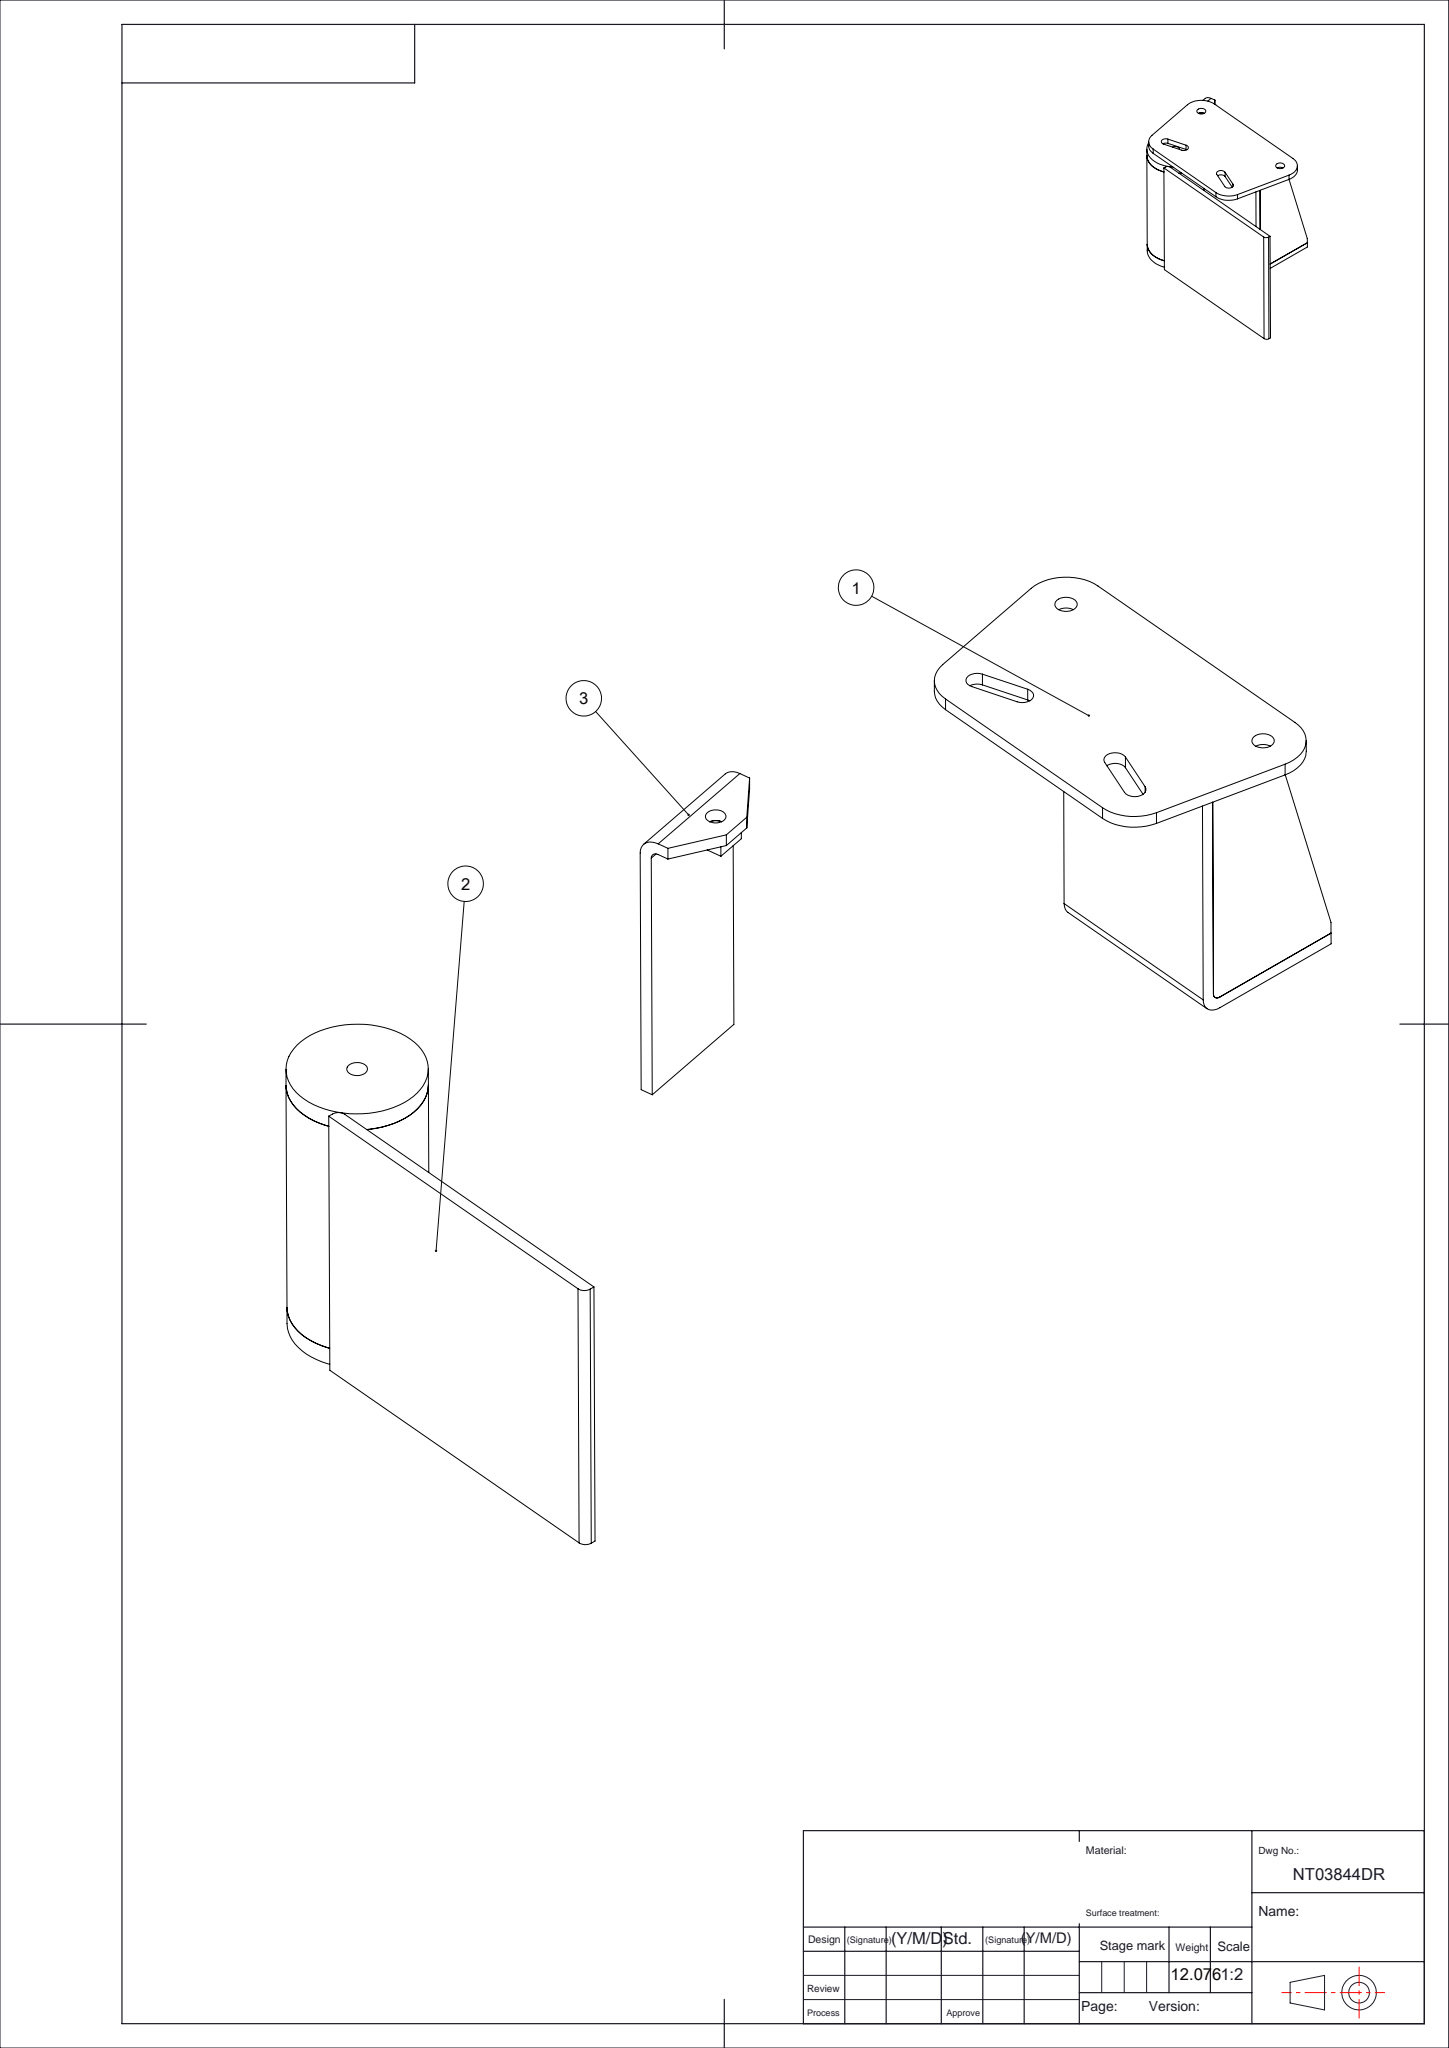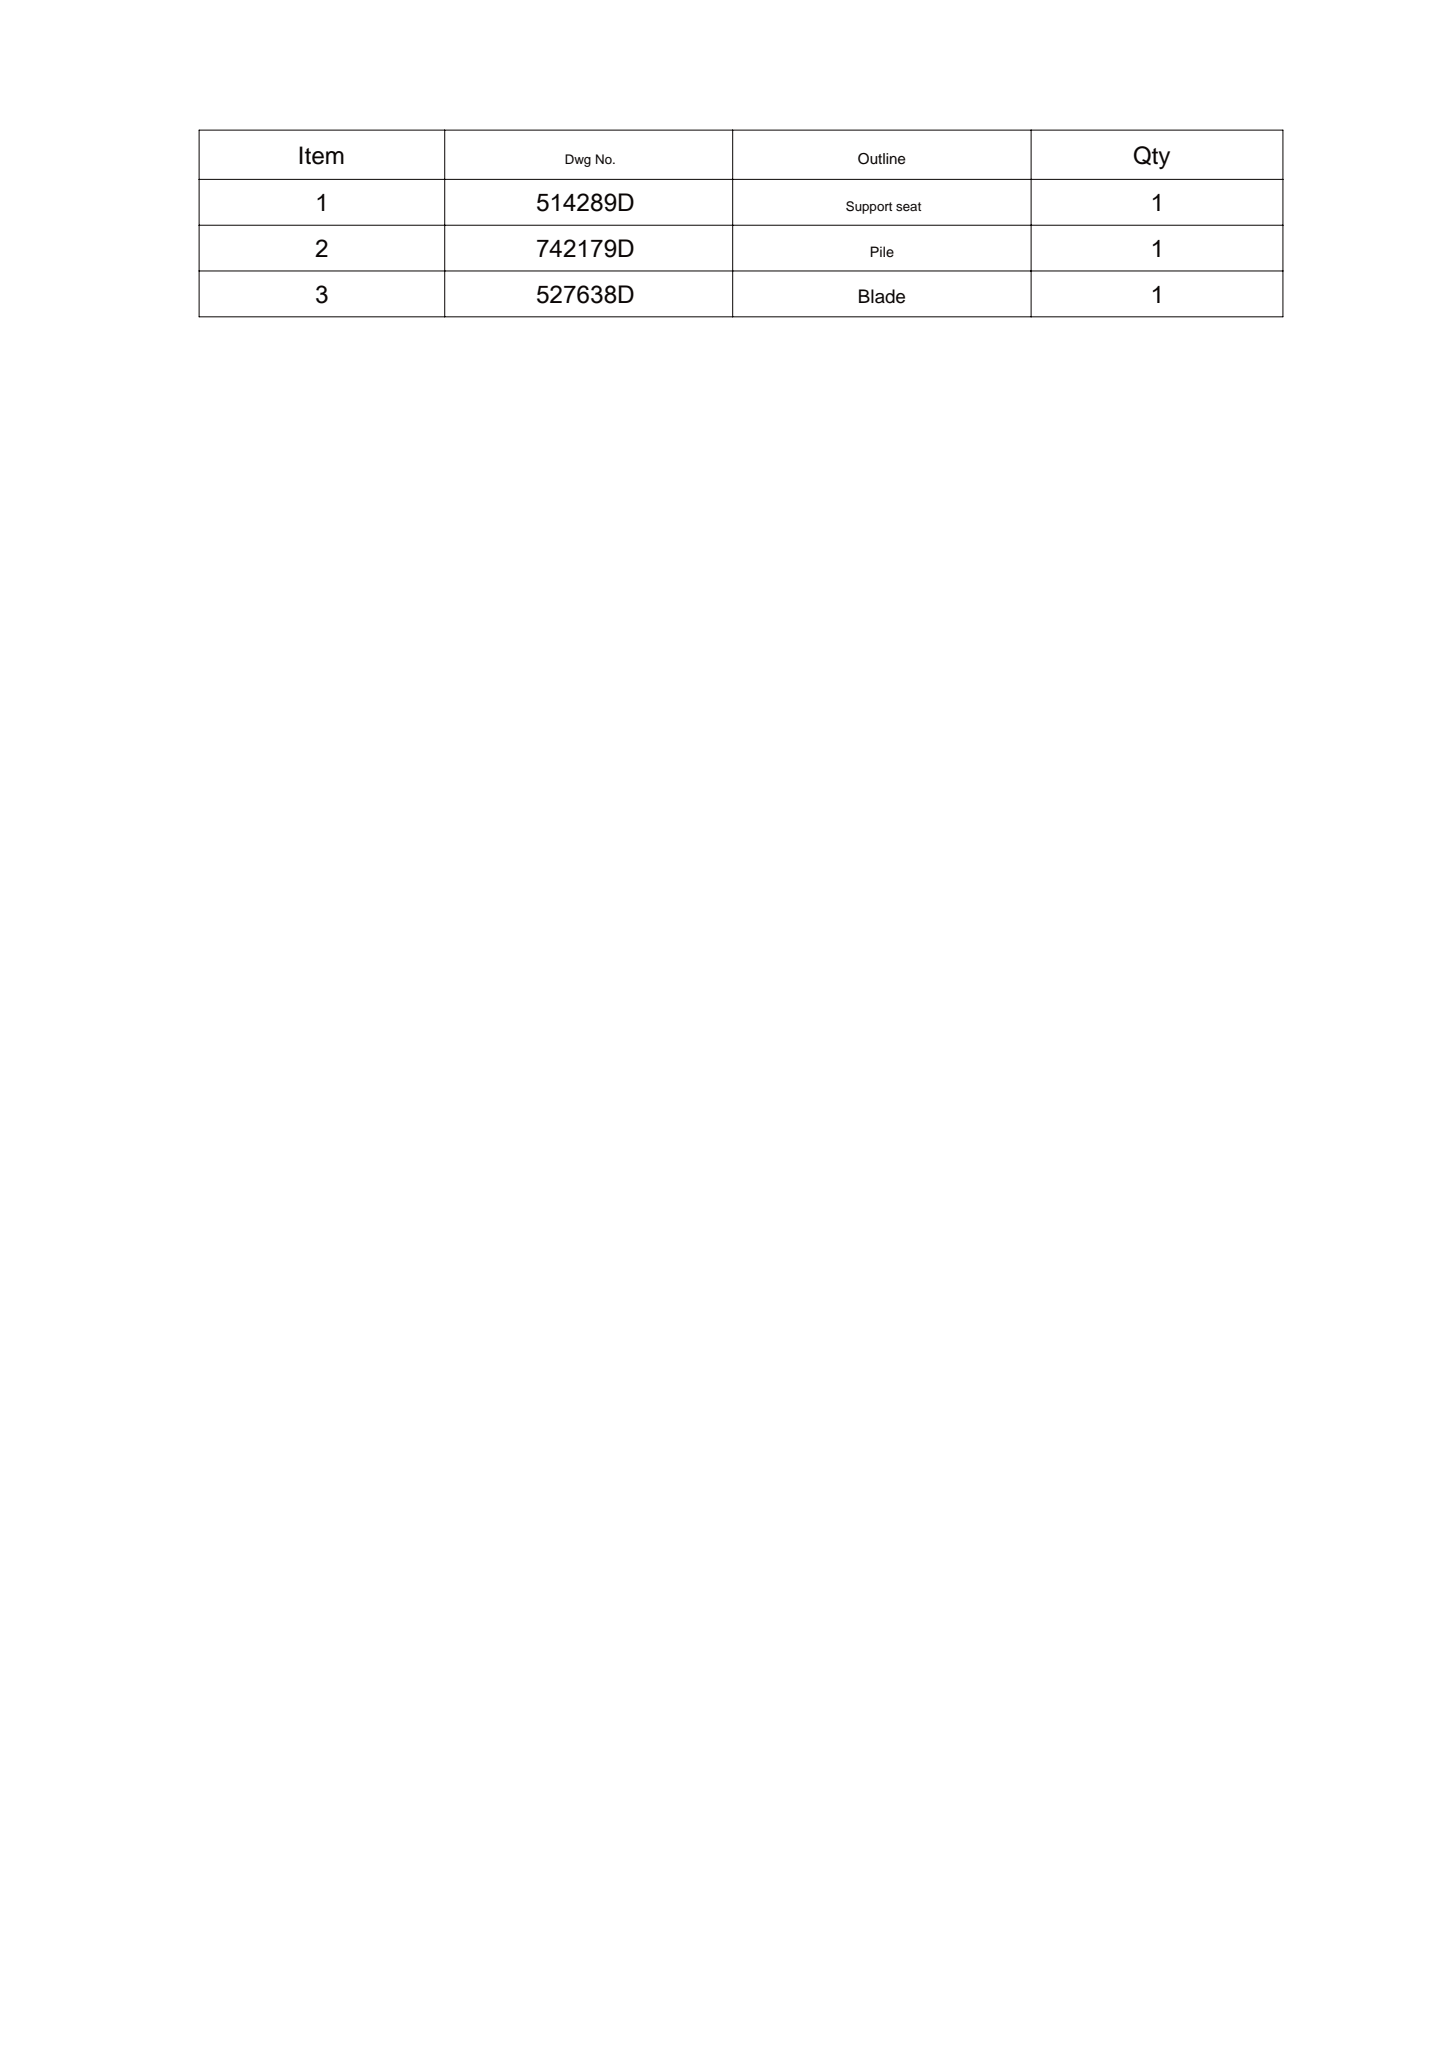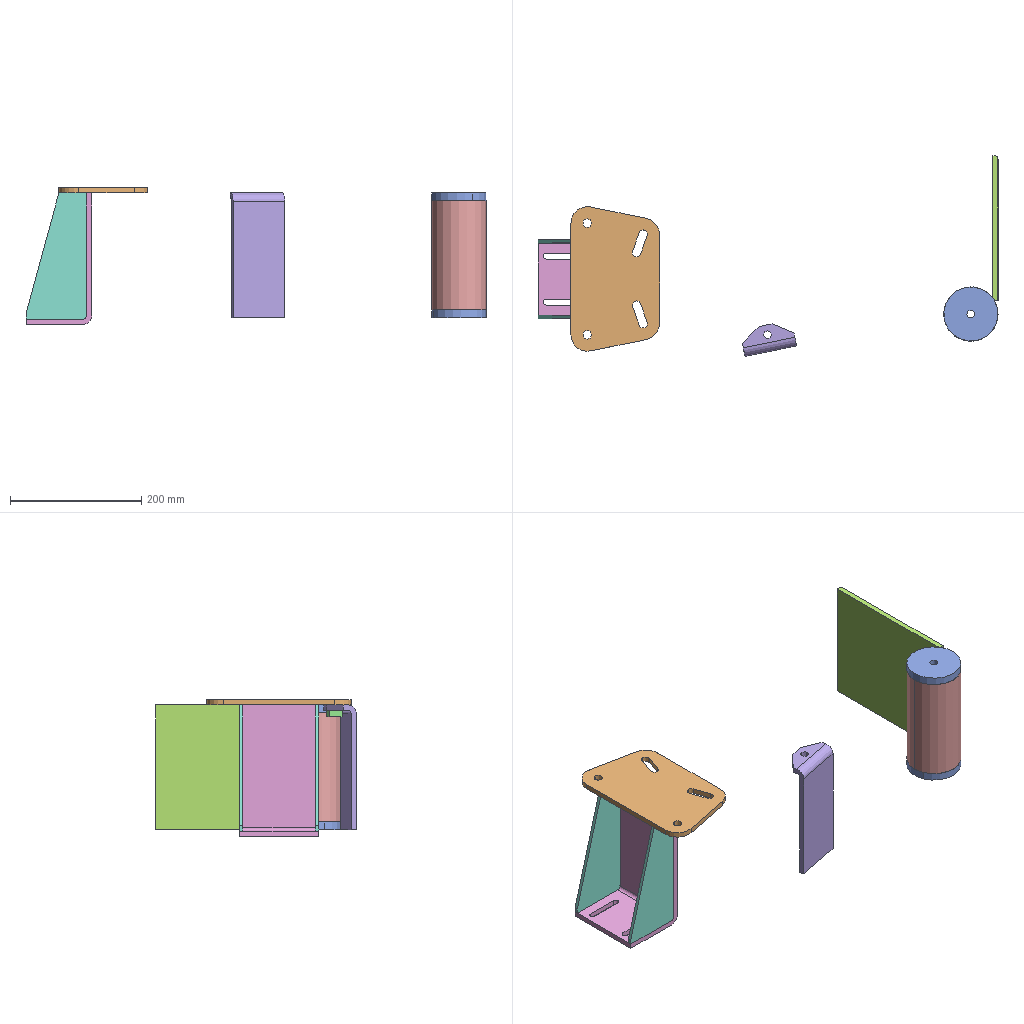Assembly | SolidWorks | 11 different items | 13 placed | box 700 x 305 x 208 mm
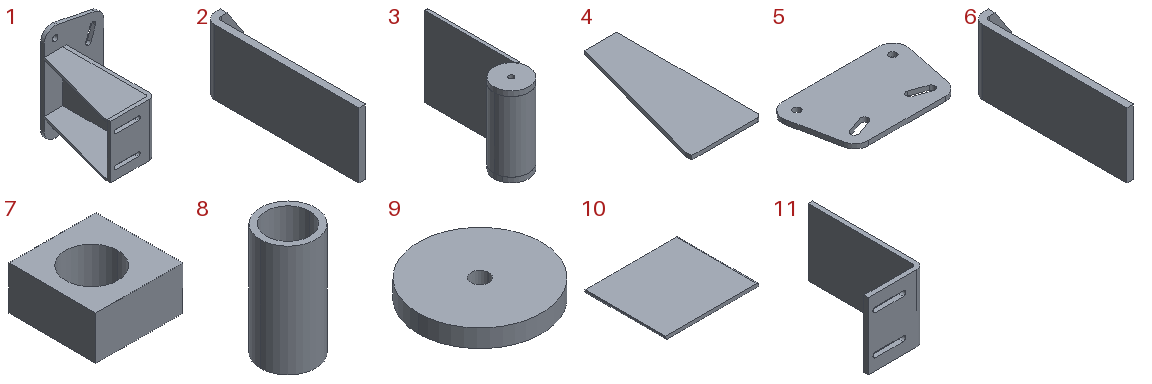Parts list (item | name | quantity | parent item | size | volume | features):
1 | (subassembly) | x1 | - | 185 x 208 x 220 mm | 603876 mm3 | -
2 | (subassembly) | x1 | - | 40 x 190 x 80 mm | 136772 mm3 | features CompositeCurve 1
3 | (subassembly) | x1 | - | 82.5 x 282.25 x 190 mm | 796169 mm3 | -
4 | - | x2 | in 1 | 92 x 192 x 5 mm | 65293 mm3 | features Extrusion 1
5 | - | x1 | in 1 | 220 x 135 x 8 mm | 204896 mm3 | features Extrusion 1
6 | - | x1 | in 2 | 40 x 190 x 80 mm | 133903 mm3 | features Extrusion 1, ICE 1
7 | - | x1 | in 2 | 20 x 20 x 10 mm | 2869 mm3 | features Extrusion 1
8 | - | x1 | in 3 | 82.5 x 82.5 x 166 mm | 338227 mm3 | features Extrusion 1
9 | - | x2 | in 3 | 82.5 x 82.5 x 12 mm | 62790 mm3 | features Extrusion 1
10 | - | x1 | in 3 | 220 x 190 x 8 mm | 332361 mm3 | features Extrusion 1, Fillet 1
11 | - | x1 | in 1 | 100 x 200 x 120 mm | 268394 mm3 | features Extrusion 1, ICE 1
Mates (type | each side: item.copy, entity, surface, feature):
In the top assembly
Coincident | 9.1 face plane Boss-Extrude1 | 5.1 face plane Boss-Extrude1
Slot | 5.1 face plane Boss-Extrude1 | 9.1 face cylinder Boss-Extrude1
Parallel | 10.1 face plane Boss-Extrude1 | 11.1 face plane Boss-Extrude1
DistanceDim | 11.1 face plane Boss-Extrude1 | 10.1 face plane Boss-Extrude1
Coincident | 5.1 face plane Boss-Extrude1 | 6.1 face plane Boss-Extrude1 | 2 times
Concentric | 5.1 edge | 6.1 edge
In subassembly 3
Coincident | 8.1 face plane Boss-Extrude1 | 9.2 face plane Boss-Extrude1
Concentric | 8.1 face cylinder Boss-Extrude1 | 9.2 face cylinder Boss-Extrude1
Concentric | 8.1 face cylinder Boss-Extrude1 | 9.3 face cylinder Boss-Extrude1
Coincident | 8.1 face plane Boss-Extrude1 | 9.3 face plane Boss-Extrude1
Parallel | 9.3 face plane Boss-Extrude1 | 10.2 face plane Boss-Extrude1
Tangent | 8.1 face cylinder Boss-Extrude1 | 10.2 face plane Boss-Extrude1
Tangent | 8.1 face cylinder Boss-Extrude1 | 10.2 face cylinder Fillet1
Width | 9.2 face plane Boss-Extrude1 | 9.3 face plane Boss-Extrude1 | 10.2 face plane Boss-Extrude1 | 10.2 face plane Boss-Extrude1
Perpendicular | 10.2 face plane Boss-Extrude1 | 3.1 plane
In subassembly 1
Coincident | 11.2 face plane Boss-Extrude1 | 4.1 face plane Boss-Extrude1 | 2 times
Coincident | 11.2 face plane Boss-Extrude1 | 4.2 face plane Boss-Extrude1 | 3 times
Coincident | 11.2 face plane Boss-Extrude1 | 4.1 edge
Coincident | 11.2 face plane Boss-Extrude1 | 5.2 face plane Boss-Extrude1
DistanceDim | 5.2 face plane Boss-Extrude1 | 11.2 face plane Boss-Extrude1
Width | 5.2 face plane Boss-Extrude1 | 5.2 face plane Boss-Extrude1 | 4.2 face plane Boss-Extrude1 | 4.1 face plane Boss-Extrude1
In subassembly 2
Coincident | 6.2 face plane Boss-Extrude1 | 7.1 face plane Boss-Extrude1
Coincident | 6.2 face cylinder Cut-Extrude1 | 7.1 edge